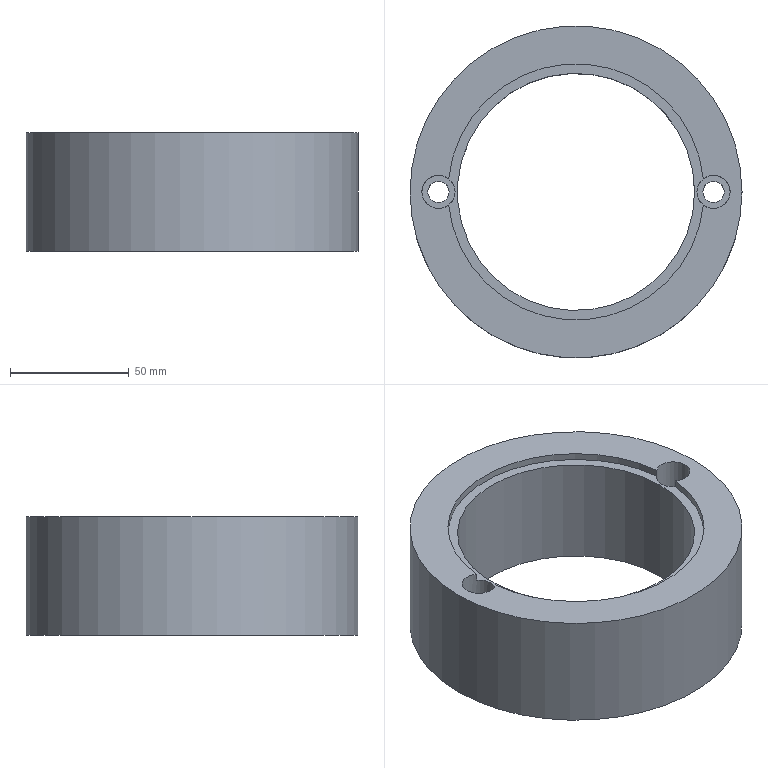Part | NX | features solid 2 | 1 solid | 13 faces | box 140 x 140 x 50 mm | volume 363234 mm3 | cylinder 8 | plane 5 | commonest cylinder face diameters 9 x2 14 x2 108 x2 100 x1 140 x1
STEP:
#1=CARTESIAN_POINT('',(-887.5,340.,-25.));
#2=VERTEX_POINT('',#1);
#3=CARTESIAN_POINT('',(-892.,340.,-25.));
#4=DIRECTION('',(0.,0.,1.));
#5=DIRECTION('',(1.,0.,0.));
#6=AXIS2_PLACEMENT_3D('',#3,#4,#5);
#7=CIRCLE('',#6,4.5);
#8=EDGE_CURVE('',#2,#2,#7,.T.);
#9=ORIENTED_EDGE('',*,*,#8,.F.);
#10=EDGE_LOOP('',(#9));
#11=FACE_BOUND('',#10,.T.);
#12=CARTESIAN_POINT('',(-887.5,340.,5.));
#13=VERTEX_POINT('',#12);
#14=CARTESIAN_POINT('',(-892.,340.,5.));
#15=DIRECTION('',(0.,0.,1.));
#16=DIRECTION('',(1.,0.,0.));
#17=AXIS2_PLACEMENT_3D('',#14,#15,#16);
#18=CIRCLE('',#17,4.5);
#19=EDGE_CURVE('',#13,#13,#18,.F.);
#20=ORIENTED_EDGE('',*,*,#19,.F.);
#21=EDGE_LOOP('',(#20));
#22=FACE_BOUND('',#21,.T.);
#23=CARTESIAN_POINT('',(-892.,340.,-75.));
#24=DIRECTION('',(0.,0.,1.));
#25=DIRECTION('',(1.,0.,0.));
#26=AXIS2_PLACEMENT_3D('',#23,#24,#25);
#27=CYLINDRICAL_SURFACE('',#26,4.5);
#28=ADVANCED_FACE('',(#11,#22),#27,.F.);
#29=CARTESIAN_POINT('',(-1003.5,340.,-25.));
#30=VERTEX_POINT('',#29);
#31=CARTESIAN_POINT('',(-1008.,340.,-25.));
#32=DIRECTION('',(0.,0.,1.));
#33=DIRECTION('',(1.,0.,0.));
#34=AXIS2_PLACEMENT_3D('',#31,#32,#33);
#35=CIRCLE('',#34,4.5);
#36=EDGE_CURVE('',#30,#30,#35,.T.);
#37=ORIENTED_EDGE('',*,*,#36,.F.);
#38=EDGE_LOOP('',(#37));
#39=FACE_BOUND('',#38,.T.);
#40=CARTESIAN_POINT('',(-1003.5,340.,5.));
#41=VERTEX_POINT('',#40);
#42=CARTESIAN_POINT('',(-1008.,340.,5.));
#43=DIRECTION('',(0.,0.,1.));
#44=DIRECTION('',(1.,0.,0.));
#45=AXIS2_PLACEMENT_3D('',#42,#43,#44);
#46=CIRCLE('',#45,4.5);
#47=EDGE_CURVE('',#41,#41,#46,.F.);
#48=ORIENTED_EDGE('',*,*,#47,.F.);
#49=EDGE_LOOP('',(#48));
#50=FACE_BOUND('',#49,.T.);
#51=CARTESIAN_POINT('',(-1008.,340.,-75.));
#52=DIRECTION('',(0.,0.,1.));
#53=DIRECTION('',(1.,0.,0.));
#54=AXIS2_PLACEMENT_3D('',#51,#52,#53);
#55=CYLINDRICAL_SURFACE('',#54,4.5);
#56=ADVANCED_FACE('',(#39,#50),#55,.F.);
#57=CARTESIAN_POINT('',(-896.284,345.536,22.));
#58=VERTEX_POINT('',#57);
#59=CARTESIAN_POINT('',(-1003.716,345.536,22.));
#60=VERTEX_POINT('',#59);
#61=CARTESIAN_POINT('',(-950.,340.,22.));
#62=DIRECTION('',(0.,0.,1.));
#63=DIRECTION('',(1.,0.,0.));
#64=AXIS2_PLACEMENT_3D('',#61,#62,#63);
#65=CIRCLE('',#64,54.);
#66=EDGE_CURVE('',#58,#60,#65,.T.);
#67=ORIENTED_EDGE('',*,*,#66,.F.);
#68=CARTESIAN_POINT('',(-896.284,345.536,25.));
#69=VERTEX_POINT('',#68);
#70=CARTESIAN_POINT('',(-896.284,345.536,15.));
#71=DIRECTION('',(0.,0.,1.));
#72=VECTOR('',#71,1000.);
#73=LINE('',#70,#72);
#74=EDGE_CURVE('',#58,#69,#73,.T.);
#75=ORIENTED_EDGE('',*,*,#74,.T.);
#76=CARTESIAN_POINT('',(-1003.716,345.536,25.));
#77=VERTEX_POINT('',#76);
#78=CARTESIAN_POINT('',(-950.,340.,25.));
#79=DIRECTION('',(0.,0.,1.));
#80=DIRECTION('',(1.,0.,0.));
#81=AXIS2_PLACEMENT_3D('',#78,#79,#80);
#82=CIRCLE('',#81,54.);
#83=EDGE_CURVE('',#69,#77,#82,.T.);
#84=ORIENTED_EDGE('',*,*,#83,.T.);
#85=CARTESIAN_POINT('',(-1003.716,345.536,15.));
#86=DIRECTION('',(0.,0.,1.));
#87=VECTOR('',#86,1000.);
#88=LINE('',#85,#87);
#89=EDGE_CURVE('',#77,#60,#88,.F.);
#90=ORIENTED_EDGE('',*,*,#89,.T.);
#91=EDGE_LOOP('',(#67,#75,#84,#90));
#92=FACE_BOUND('',#91,.T.);
#93=CARTESIAN_POINT('',(-950.,340.,22.));
#94=DIRECTION('',(0.,0.,1.));
#95=DIRECTION('',(1.,0.,0.));
#96=AXIS2_PLACEMENT_3D('',#93,#94,#95);
#97=CYLINDRICAL_SURFACE('',#96,54.);
#98=ADVANCED_FACE('',(#92),#97,.F.);
#99=CARTESIAN_POINT('',(-900.,340.,-25.));
#100=VERTEX_POINT('',#99);
#101=CARTESIAN_POINT('',(-950.,340.,-25.));
#102=DIRECTION('',(0.,0.,1.));
#103=DIRECTION('',(1.,0.,0.));
#104=AXIS2_PLACEMENT_3D('',#101,#102,#103);
#105=CIRCLE('',#104,50.);
#106=EDGE_CURVE('',#100,#100,#105,.T.);
#107=ORIENTED_EDGE('',*,*,#106,.F.);
#108=EDGE_LOOP('',(#107));
#109=FACE_BOUND('',#108,.T.);
#110=CARTESIAN_POINT('',(-900.,340.,22.));
#111=VERTEX_POINT('',#110);
#112=CARTESIAN_POINT('',(-950.,340.,22.));
#113=DIRECTION('',(0.,0.,1.));
#114=DIRECTION('',(1.,0.,0.));
#115=AXIS2_PLACEMENT_3D('',#112,#113,#114);
#116=CIRCLE('',#115,50.);
#117=EDGE_CURVE('',#111,#111,#116,.T.);
#118=ORIENTED_EDGE('',*,*,#117,.T.);
#119=EDGE_LOOP('',(#118));
#120=FACE_BOUND('',#119,.T.);
#121=CARTESIAN_POINT('',(-950.,340.,25.));
#122=DIRECTION('',(0.,0.,-1.));
#123=DIRECTION('',(-1.,0.,0.));
#124=AXIS2_PLACEMENT_3D('',#121,#122,#123);
#125=CYLINDRICAL_SURFACE('',#124,50.);
#126=ADVANCED_FACE('',(#109,#120),#125,.F.);
#127=CARTESIAN_POINT('',(-880.,340.,25.));
#128=VERTEX_POINT('',#127);
#129=CARTESIAN_POINT('',(-950.,340.,25.));
#130=DIRECTION('',(0.,0.,1.));
#131=DIRECTION('',(1.,0.,0.));
#132=AXIS2_PLACEMENT_3D('',#129,#130,#131);
#133=CIRCLE('',#132,70.);
#134=EDGE_CURVE('',#128,#128,#133,.T.);
#135=ORIENTED_EDGE('',*,*,#134,.F.);
#136=EDGE_LOOP('',(#135));
#137=FACE_BOUND('',#136,.T.);
#138=CARTESIAN_POINT('',(-880.,340.,-25.));
#139=VERTEX_POINT('',#138);
#140=CARTESIAN_POINT('',(-950.,340.,-25.));
#141=DIRECTION('',(0.,0.,1.));
#142=DIRECTION('',(1.,0.,0.));
#143=AXIS2_PLACEMENT_3D('',#140,#141,#142);
#144=CIRCLE('',#143,70.);
#145=EDGE_CURVE('',#139,#139,#144,.T.);
#146=ORIENTED_EDGE('',*,*,#145,.T.);
#147=EDGE_LOOP('',(#146));
#148=FACE_BOUND('',#147,.T.);
#149=CARTESIAN_POINT('',(-950.,340.,25.));
#150=DIRECTION('',(0.,0.,-1.));
#151=DIRECTION('',(-1.,0.,0.));
#152=AXIS2_PLACEMENT_3D('',#149,#150,#151);
#153=CYLINDRICAL_SURFACE('',#152,70.);
#154=ADVANCED_FACE('',(#137,#148),#153,.T.);
#155=CARTESIAN_POINT('',(-896.284,334.464,25.));
#156=VERTEX_POINT('',#155);
#157=CARTESIAN_POINT('',(-892.,340.,25.));
#158=DIRECTION('',(0.,0.,1.));
#159=DIRECTION('',(1.,0.,0.));
#160=AXIS2_PLACEMENT_3D('',#157,#158,#159);
#161=CIRCLE('',#160,7.);
#162=EDGE_CURVE('',#156,#69,#161,.T.);
#163=ORIENTED_EDGE('',*,*,#162,.F.);
#164=CARTESIAN_POINT('',(-1003.716,334.464,25.));
#165=VERTEX_POINT('',#164);
#166=CARTESIAN_POINT('',(-950.,340.,25.));
#167=DIRECTION('',(0.,0.,1.));
#168=DIRECTION('',(1.,0.,0.));
#169=AXIS2_PLACEMENT_3D('',#166,#167,#168);
#170=CIRCLE('',#169,54.);
#171=EDGE_CURVE('',#165,#156,#170,.T.);
#172=ORIENTED_EDGE('',*,*,#171,.F.);
#173=CARTESIAN_POINT('',(-1008.,340.,25.));
#174=DIRECTION('',(0.,0.,1.));
#175=DIRECTION('',(1.,0.,0.));
#176=AXIS2_PLACEMENT_3D('',#173,#174,#175);
#177=CIRCLE('',#176,7.);
#178=EDGE_CURVE('',#77,#165,#177,.T.);
#179=ORIENTED_EDGE('',*,*,#178,.F.);
#180=ORIENTED_EDGE('',*,*,#83,.F.);
#181=EDGE_LOOP('',(#163,#172,#179,#180));
#182=FACE_BOUND('',#181,.T.);
#183=ORIENTED_EDGE('',*,*,#134,.T.);
#184=EDGE_LOOP('',(#183));
#185=FACE_BOUND('',#184,.T.);
#186=CARTESIAN_POINT('',(-950.,340.,25.));
#187=DIRECTION('',(0.,0.,1.));
#188=DIRECTION('',(1.,0.,0.));
#189=AXIS2_PLACEMENT_3D('',#186,#187,#188);
#190=PLANE('',#189);
#191=ADVANCED_FACE('',(#182,#185),#190,.T.);
#192=ORIENTED_EDGE('',*,*,#8,.T.);
#193=EDGE_LOOP('',(#192));
#194=FACE_BOUND('',#193,.T.);
#195=ORIENTED_EDGE('',*,*,#36,.T.);
#196=EDGE_LOOP('',(#195));
#197=FACE_BOUND('',#196,.T.);
#198=ORIENTED_EDGE('',*,*,#106,.T.);
#199=EDGE_LOOP('',(#198));
#200=FACE_BOUND('',#199,.T.);
#201=ORIENTED_EDGE('',*,*,#145,.F.);
#202=EDGE_LOOP('',(#201));
#203=FACE_BOUND('',#202,.T.);
#204=CARTESIAN_POINT('',(-950.,340.,-25.));
#205=DIRECTION('',(0.,0.,1.));
#206=DIRECTION('',(1.,0.,0.));
#207=AXIS2_PLACEMENT_3D('',#204,#205,#206);
#208=PLANE('',#207);
#209=ADVANCED_FACE('',(#194,#197,#200,#203),#208,.F.);
#210=ORIENTED_EDGE('',*,*,#171,.T.);
#211=CARTESIAN_POINT('',(-896.284,334.464,22.));
#212=VERTEX_POINT('',#211);
#213=CARTESIAN_POINT('',(-896.284,334.464,15.));
#214=DIRECTION('',(0.,0.,1.));
#215=VECTOR('',#214,1000.);
#216=LINE('',#213,#215);
#217=EDGE_CURVE('',#156,#212,#216,.F.);
#218=ORIENTED_EDGE('',*,*,#217,.T.);
#219=CARTESIAN_POINT('',(-1003.716,334.464,22.));
#220=VERTEX_POINT('',#219);
#221=CARTESIAN_POINT('',(-950.,340.,22.));
#222=DIRECTION('',(0.,0.,1.));
#223=DIRECTION('',(1.,0.,0.));
#224=AXIS2_PLACEMENT_3D('',#221,#222,#223);
#225=CIRCLE('',#224,54.);
#226=EDGE_CURVE('',#220,#212,#225,.T.);
#227=ORIENTED_EDGE('',*,*,#226,.F.);
#228=CARTESIAN_POINT('',(-1003.716,334.464,15.));
#229=DIRECTION('',(0.,0.,1.));
#230=VECTOR('',#229,1000.);
#231=LINE('',#228,#230);
#232=EDGE_CURVE('',#220,#165,#231,.T.);
#233=ORIENTED_EDGE('',*,*,#232,.T.);
#234=EDGE_LOOP('',(#210,#218,#227,#233));
#235=FACE_BOUND('',#234,.T.);
#236=CARTESIAN_POINT('',(-950.,340.,22.));
#237=DIRECTION('',(0.,0.,1.));
#238=DIRECTION('',(1.,0.,0.));
#239=AXIS2_PLACEMENT_3D('',#236,#237,#238);
#240=CYLINDRICAL_SURFACE('',#239,54.);
#241=ADVANCED_FACE('',(#235),#240,.F.);
#242=CARTESIAN_POINT('',(-892.,340.,22.));
#243=DIRECTION('',(0.,0.,1.));
#244=DIRECTION('',(1.,0.,0.));
#245=AXIS2_PLACEMENT_3D('',#242,#243,#244);
#246=CIRCLE('',#245,7.);
#247=EDGE_CURVE('',#58,#212,#246,.T.);
#248=ORIENTED_EDGE('',*,*,#247,.F.);
#249=ORIENTED_EDGE('',*,*,#66,.T.);
#250=CARTESIAN_POINT('',(-1008.,340.,22.));
#251=DIRECTION('',(0.,0.,1.));
#252=DIRECTION('',(1.,0.,0.));
#253=AXIS2_PLACEMENT_3D('',#250,#251,#252);
#254=CIRCLE('',#253,7.);
#255=EDGE_CURVE('',#220,#60,#254,.T.);
#256=ORIENTED_EDGE('',*,*,#255,.F.);
#257=ORIENTED_EDGE('',*,*,#226,.T.);
#258=EDGE_LOOP('',(#248,#249,#256,#257));
#259=FACE_BOUND('',#258,.T.);
#260=ORIENTED_EDGE('',*,*,#117,.F.);
#261=EDGE_LOOP('',(#260));
#262=FACE_BOUND('',#261,.T.);
#263=CARTESIAN_POINT('',(-950.,340.,22.));
#264=DIRECTION('',(0.,0.,1.));
#265=DIRECTION('',(1.,0.,0.));
#266=AXIS2_PLACEMENT_3D('',#263,#264,#265);
#267=PLANE('',#266);
#268=ADVANCED_FACE('',(#259,#262),#267,.T.);
#269=CARTESIAN_POINT('',(-1001.,340.,5.));
#270=VERTEX_POINT('',#269);
#271=CARTESIAN_POINT('',(-1008.,340.,5.));
#272=DIRECTION('',(0.,0.,1.));
#273=DIRECTION('',(1.,0.,0.));
#274=AXIS2_PLACEMENT_3D('',#271,#272,#273);
#275=CIRCLE('',#274,7.);
#276=EDGE_CURVE('',#270,#270,#275,.T.);
#277=ORIENTED_EDGE('',*,*,#276,.F.);
#278=EDGE_LOOP('',(#277));
#279=FACE_BOUND('',#278,.T.);
#280=ORIENTED_EDGE('',*,*,#178,.T.);
#281=ORIENTED_EDGE('',*,*,#232,.F.);
#282=ORIENTED_EDGE('',*,*,#255,.T.);
#283=ORIENTED_EDGE('',*,*,#89,.F.);
#284=EDGE_LOOP('',(#280,#281,#282,#283));
#285=FACE_BOUND('',#284,.T.);
#286=CARTESIAN_POINT('',(-1008.,340.,5.));
#287=DIRECTION('',(0.,0.,1.));
#288=DIRECTION('',(1.,0.,0.));
#289=AXIS2_PLACEMENT_3D('',#286,#287,#288);
#290=CYLINDRICAL_SURFACE('',#289,7.);
#291=ADVANCED_FACE('',(#279,#285),#290,.F.);
#292=ORIENTED_EDGE('',*,*,#276,.T.);
#293=EDGE_LOOP('',(#292));
#294=FACE_BOUND('',#293,.T.);
#295=ORIENTED_EDGE('',*,*,#47,.T.);
#296=EDGE_LOOP('',(#295));
#297=FACE_BOUND('',#296,.T.);
#298=CARTESIAN_POINT('',(-1008.,340.,5.));
#299=DIRECTION('',(0.,0.,1.));
#300=DIRECTION('',(1.,0.,0.));
#301=AXIS2_PLACEMENT_3D('',#298,#299,#300);
#302=PLANE('',#301);
#303=ADVANCED_FACE('',(#294,#297),#302,.T.);
#304=CARTESIAN_POINT('',(-885.,340.,5.));
#305=VERTEX_POINT('',#304);
#306=CARTESIAN_POINT('',(-892.,340.,5.));
#307=DIRECTION('',(0.,0.,1.));
#308=DIRECTION('',(1.,0.,0.));
#309=AXIS2_PLACEMENT_3D('',#306,#307,#308);
#310=CIRCLE('',#309,7.);
#311=EDGE_CURVE('',#305,#305,#310,.T.);
#312=ORIENTED_EDGE('',*,*,#311,.F.);
#313=EDGE_LOOP('',(#312));
#314=FACE_BOUND('',#313,.T.);
#315=ORIENTED_EDGE('',*,*,#247,.T.);
#316=ORIENTED_EDGE('',*,*,#217,.F.);
#317=ORIENTED_EDGE('',*,*,#162,.T.);
#318=ORIENTED_EDGE('',*,*,#74,.F.);
#319=EDGE_LOOP('',(#315,#316,#317,#318));
#320=FACE_BOUND('',#319,.T.);
#321=CARTESIAN_POINT('',(-892.,340.,5.));
#322=DIRECTION('',(0.,0.,1.));
#323=DIRECTION('',(1.,0.,0.));
#324=AXIS2_PLACEMENT_3D('',#321,#322,#323);
#325=CYLINDRICAL_SURFACE('',#324,7.);
#326=ADVANCED_FACE('',(#314,#320),#325,.F.);
#327=ORIENTED_EDGE('',*,*,#311,.T.);
#328=EDGE_LOOP('',(#327));
#329=FACE_BOUND('',#328,.T.);
#330=ORIENTED_EDGE('',*,*,#19,.T.);
#331=EDGE_LOOP('',(#330));
#332=FACE_BOUND('',#331,.T.);
#333=CARTESIAN_POINT('',(-892.,340.,5.));
#334=DIRECTION('',(0.,0.,1.));
#335=DIRECTION('',(1.,0.,0.));
#336=AXIS2_PLACEMENT_3D('',#333,#334,#335);
#337=PLANE('',#336);
#338=ADVANCED_FACE('',(#329,#332),#337,.T.);
#339=CLOSED_SHELL('',(#28,#56,#98,#126,#154,#191,#209,#241,#268,#291,#303,#326,#338));
#340=MANIFOLD_SOLID_BREP('',#339);
#341=(LENGTH_UNIT()NAMED_UNIT(*)SI_UNIT(.MILLI.,.METRE.));
#342=UNCERTAINTY_MEASURE_WITH_UNIT(LENGTH_MEASURE(0.00001),#341,'','');
#343=(NAMED_UNIT(*)PLANE_ANGLE_UNIT()SI_UNIT($,.RADIAN.));
#344=(NAMED_UNIT(*)SI_UNIT($,.STERADIAN.)SOLID_ANGLE_UNIT());
#345=(GEOMETRIC_REPRESENTATION_CONTEXT(3)GLOBAL_UNCERTAINTY_ASSIGNED_CONTEXT((#342))GLOBAL_UNIT_ASSIGNED_CONTEXT((#341,#343,#344))REPRESENTATION_CONTEXT('',''));
#346=ADVANCED_BREP_SHAPE_REPRESENTATION('',(#340),#345);